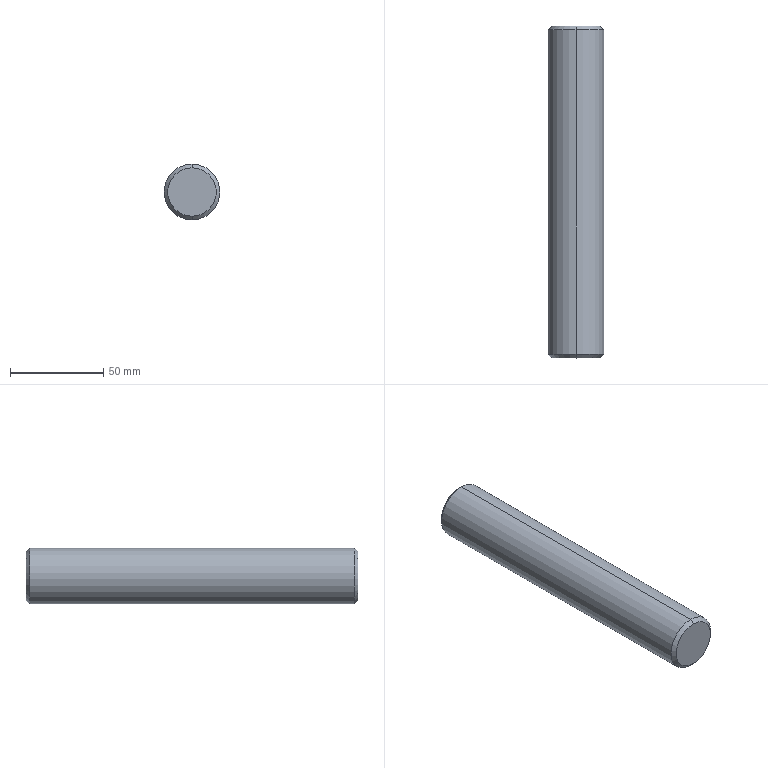Part | SolidWorks | features Chamfer 1, Revolution 1 | 1 solid | 8 faces | box 30 x 178 x 30 mm | volume 125461 mm3 | cone 4 | cylinder 2 | plane 2 | commonest cylinder face diameters 30 x2
STEP:
#1=CARTESIAN_POINT('',(0.,178.,13.));
#2=VERTEX_POINT('',#1);
#3=CARTESIAN_POINT('',(0.,178.,-13.));
#4=VERTEX_POINT('',#3);
#5=CARTESIAN_POINT('',(0.,178.,0.));
#6=DIRECTION('',(0.,1.,0.));
#7=DIRECTION('',(0.,0.,1.));
#8=AXIS2_PLACEMENT_3D('',#5,#6,#7);
#9=CIRCLE('',#8,13.);
#10=EDGE_CURVE('',#2,#4,#9,.T.);
#11=ORIENTED_EDGE('',*,*,#10,.F.);
#12=CARTESIAN_POINT('',(0.,176.,15.));
#13=VERTEX_POINT('',#12);
#14=CARTESIAN_POINT('',(0.,176.,15.));
#15=DIRECTION('',(0.,-0.7071,0.7071));
#16=VECTOR('',#15,1000.);
#17=LINE('',#14,#16);
#18=EDGE_CURVE('',#2,#13,#17,.T.);
#19=ORIENTED_EDGE('',*,*,#18,.T.);
#20=CARTESIAN_POINT('',(0.,176.,-15.));
#21=VERTEX_POINT('',#20);
#22=CARTESIAN_POINT('',(0.,176.,0.));
#23=DIRECTION('',(0.,-1.,0.));
#24=DIRECTION('',(0.,0.,1.));
#25=AXIS2_PLACEMENT_3D('',#22,#23,#24);
#26=CIRCLE('',#25,15.);
#27=EDGE_CURVE('',#21,#13,#26,.T.);
#28=ORIENTED_EDGE('',*,*,#27,.F.);
#29=CARTESIAN_POINT('',(0.,176.,-15.));
#30=DIRECTION('',(0.,-0.7071,-0.7071));
#31=VECTOR('',#30,1000.);
#32=LINE('',#29,#31);
#33=EDGE_CURVE('',#4,#21,#32,.T.);
#34=ORIENTED_EDGE('',*,*,#33,.F.);
#35=EDGE_LOOP('',(#11,#19,#28,#34));
#36=FACE_OUTER_BOUND('',#35,.T.);
#37=CARTESIAN_POINT('',(0.,176.,0.));
#38=DIRECTION('',(0.,-1.,0.));
#39=DIRECTION('',(0.,0.,-1.));
#40=AXIS2_PLACEMENT_3D('',#37,#38,#39);
#41=CONICAL_SURFACE('',#40,15.,0.7854);
#42=ADVANCED_FACE('',(#36),#41,.T.);
#43=CARTESIAN_POINT('',(0.,0.,-13.));
#44=VERTEX_POINT('',#43);
#45=CARTESIAN_POINT('',(0.,0.,13.));
#46=VERTEX_POINT('',#45);
#47=CARTESIAN_POINT('',(0.,0.,0.));
#48=DIRECTION('',(0.,-1.,0.));
#49=DIRECTION('',(0.,0.,-1.));
#50=AXIS2_PLACEMENT_3D('',#47,#48,#49);
#51=CIRCLE('',#50,13.);
#52=EDGE_CURVE('',#44,#46,#51,.T.);
#53=ORIENTED_EDGE('',*,*,#52,.F.);
#54=CARTESIAN_POINT('',(0.,2.,-15.));
#55=VERTEX_POINT('',#54);
#56=CARTESIAN_POINT('',(0.,0.,-13.));
#57=DIRECTION('',(0.,0.7071,-0.7071));
#58=VECTOR('',#57,1000.);
#59=LINE('',#56,#58);
#60=EDGE_CURVE('',#44,#55,#59,.T.);
#61=ORIENTED_EDGE('',*,*,#60,.T.);
#62=CARTESIAN_POINT('',(0.,2.,15.));
#63=VERTEX_POINT('',#62);
#64=CARTESIAN_POINT('',(0.,2.,0.));
#65=DIRECTION('',(0.,1.,0.));
#66=DIRECTION('',(0.,0.,-1.));
#67=AXIS2_PLACEMENT_3D('',#64,#65,#66);
#68=CIRCLE('',#67,15.);
#69=EDGE_CURVE('',#63,#55,#68,.T.);
#70=ORIENTED_EDGE('',*,*,#69,.F.);
#71=CARTESIAN_POINT('',(0.,0.,13.));
#72=DIRECTION('',(0.,0.7071,0.7071));
#73=VECTOR('',#72,1000.);
#74=LINE('',#71,#73);
#75=EDGE_CURVE('',#46,#63,#74,.T.);
#76=ORIENTED_EDGE('',*,*,#75,.F.);
#77=EDGE_LOOP('',(#53,#61,#70,#76));
#78=FACE_OUTER_BOUND('',#77,.T.);
#79=CARTESIAN_POINT('',(0.,0.,0.));
#80=DIRECTION('',(0.,1.,0.));
#81=DIRECTION('',(0.,0.,1.));
#82=AXIS2_PLACEMENT_3D('',#79,#80,#81);
#83=CONICAL_SURFACE('',#82,13.,0.7854);
#84=ADVANCED_FACE('',(#78),#83,.T.);
#85=ORIENTED_EDGE('',*,*,#27,.T.);
#86=CARTESIAN_POINT('',(0.,0.,15.));
#87=DIRECTION('',(0.,-1.,0.));
#88=VECTOR('',#87,1000.);
#89=LINE('',#86,#88);
#90=EDGE_CURVE('',#13,#63,#89,.T.);
#91=ORIENTED_EDGE('',*,*,#90,.T.);
#92=ORIENTED_EDGE('',*,*,#69,.T.);
#93=CARTESIAN_POINT('',(0.,0.,-15.));
#94=DIRECTION('',(0.,-1.,0.));
#95=VECTOR('',#94,1000.);
#96=LINE('',#93,#95);
#97=EDGE_CURVE('',#21,#55,#96,.T.);
#98=ORIENTED_EDGE('',*,*,#97,.F.);
#99=EDGE_LOOP('',(#85,#91,#92,#98));
#100=FACE_OUTER_BOUND('',#99,.T.);
#101=CARTESIAN_POINT('',(0.,0.,0.));
#102=DIRECTION('',(0.,-1.,0.));
#103=DIRECTION('',(0.,0.,-1.));
#104=AXIS2_PLACEMENT_3D('',#101,#102,#103);
#105=CYLINDRICAL_SURFACE('',#104,15.);
#106=ADVANCED_FACE('',(#100),#105,.T.);
#107=CARTESIAN_POINT('',(0.,0.,0.));
#108=DIRECTION('',(0.,-1.,0.));
#109=DIRECTION('',(0.,0.,-1.));
#110=AXIS2_PLACEMENT_3D('',#107,#108,#109);
#111=CIRCLE('',#110,13.);
#112=EDGE_CURVE('',#46,#44,#111,.T.);
#113=ORIENTED_EDGE('',*,*,#112,.T.);
#114=ORIENTED_EDGE('',*,*,#52,.T.);
#115=EDGE_LOOP('',(#113,#114));
#116=FACE_OUTER_BOUND('',#115,.T.);
#117=CARTESIAN_POINT('',(0.,0.,0.));
#118=DIRECTION('',(0.,-1.,0.));
#119=DIRECTION('',(0.,0.,-1.));
#120=AXIS2_PLACEMENT_3D('',#117,#118,#119);
#121=PLANE('',#120);
#122=ADVANCED_FACE('',(#116),#121,.T.);
#123=ORIENTED_EDGE('',*,*,#90,.F.);
#124=CARTESIAN_POINT('',(0.,176.,0.));
#125=DIRECTION('',(0.,-1.,0.));
#126=DIRECTION('',(0.,0.,1.));
#127=AXIS2_PLACEMENT_3D('',#124,#125,#126);
#128=CIRCLE('',#127,15.);
#129=EDGE_CURVE('',#13,#21,#128,.T.);
#130=ORIENTED_EDGE('',*,*,#129,.T.);
#131=ORIENTED_EDGE('',*,*,#97,.T.);
#132=CARTESIAN_POINT('',(0.,2.,0.));
#133=DIRECTION('',(0.,1.,0.));
#134=DIRECTION('',(0.,0.,-1.));
#135=AXIS2_PLACEMENT_3D('',#132,#133,#134);
#136=CIRCLE('',#135,15.);
#137=EDGE_CURVE('',#55,#63,#136,.T.);
#138=ORIENTED_EDGE('',*,*,#137,.T.);
#139=EDGE_LOOP('',(#123,#130,#131,#138));
#140=FACE_OUTER_BOUND('',#139,.T.);
#141=CARTESIAN_POINT('',(0.,0.,0.));
#142=DIRECTION('',(0.,-1.,0.));
#143=DIRECTION('',(0.,0.,-1.));
#144=AXIS2_PLACEMENT_3D('',#141,#142,#143);
#145=CYLINDRICAL_SURFACE('',#144,15.);
#146=ADVANCED_FACE('',(#140),#145,.T.);
#147=CARTESIAN_POINT('',(0.,178.,0.));
#148=DIRECTION('',(0.,1.,0.));
#149=DIRECTION('',(0.,0.,1.));
#150=AXIS2_PLACEMENT_3D('',#147,#148,#149);
#151=CIRCLE('',#150,13.);
#152=EDGE_CURVE('',#4,#2,#151,.T.);
#153=ORIENTED_EDGE('',*,*,#152,.T.);
#154=ORIENTED_EDGE('',*,*,#10,.T.);
#155=EDGE_LOOP('',(#153,#154));
#156=FACE_OUTER_BOUND('',#155,.T.);
#157=CARTESIAN_POINT('',(15.,178.,0.));
#158=DIRECTION('',(0.,1.,0.));
#159=DIRECTION('',(0.,0.,1.));
#160=AXIS2_PLACEMENT_3D('',#157,#158,#159);
#161=PLANE('',#160);
#162=ADVANCED_FACE('',(#156),#161,.T.);
#163=ORIENTED_EDGE('',*,*,#60,.F.);
#164=ORIENTED_EDGE('',*,*,#112,.F.);
#165=ORIENTED_EDGE('',*,*,#75,.T.);
#166=ORIENTED_EDGE('',*,*,#137,.F.);
#167=EDGE_LOOP('',(#163,#164,#165,#166));
#168=FACE_OUTER_BOUND('',#167,.T.);
#169=CARTESIAN_POINT('',(0.,0.,0.));
#170=DIRECTION('',(0.,1.,0.));
#171=DIRECTION('',(0.,0.,1.));
#172=AXIS2_PLACEMENT_3D('',#169,#170,#171);
#173=CONICAL_SURFACE('',#172,13.,0.7854);
#174=ADVANCED_FACE('',(#168),#173,.T.);
#175=ORIENTED_EDGE('',*,*,#18,.F.);
#176=ORIENTED_EDGE('',*,*,#152,.F.);
#177=ORIENTED_EDGE('',*,*,#33,.T.);
#178=ORIENTED_EDGE('',*,*,#129,.F.);
#179=EDGE_LOOP('',(#175,#176,#177,#178));
#180=FACE_OUTER_BOUND('',#179,.T.);
#181=CARTESIAN_POINT('',(0.,176.,0.));
#182=DIRECTION('',(0.,-1.,0.));
#183=DIRECTION('',(0.,0.,-1.));
#184=AXIS2_PLACEMENT_3D('',#181,#182,#183);
#185=CONICAL_SURFACE('',#184,15.,0.7854);
#186=ADVANCED_FACE('',(#180),#185,.T.);
#187=CLOSED_SHELL('',(#42,#84,#106,#122,#146,#162,#174,#186));
#188=MANIFOLD_SOLID_BREP('',#187);
#189=CARTESIAN_POINT('',(0.,0.,0.));
#190=DIRECTION('',(0.,0.,1.));
#191=DIRECTION('',(1.,0.,0.));
#192=AXIS2_PLACEMENT_3D('',#189,#190,#191);
#193=(LENGTH_UNIT()NAMED_UNIT(*)SI_UNIT(.MILLI.,.METRE.));
#194=UNCERTAINTY_MEASURE_WITH_UNIT(LENGTH_MEASURE(0.00001),#193,'','');
#195=(NAMED_UNIT(*)PLANE_ANGLE_UNIT()SI_UNIT($,.RADIAN.));
#196=(NAMED_UNIT(*)SI_UNIT($,.STERADIAN.)SOLID_ANGLE_UNIT());
#197=(GEOMETRIC_REPRESENTATION_CONTEXT(3)GLOBAL_UNCERTAINTY_ASSIGNED_CONTEXT((#194))GLOBAL_UNIT_ASSIGNED_CONTEXT((#193,#195,#196))REPRESENTATION_CONTEXT('',''));
#198=ADVANCED_BREP_SHAPE_REPRESENTATION('',(#188,#192),#197);